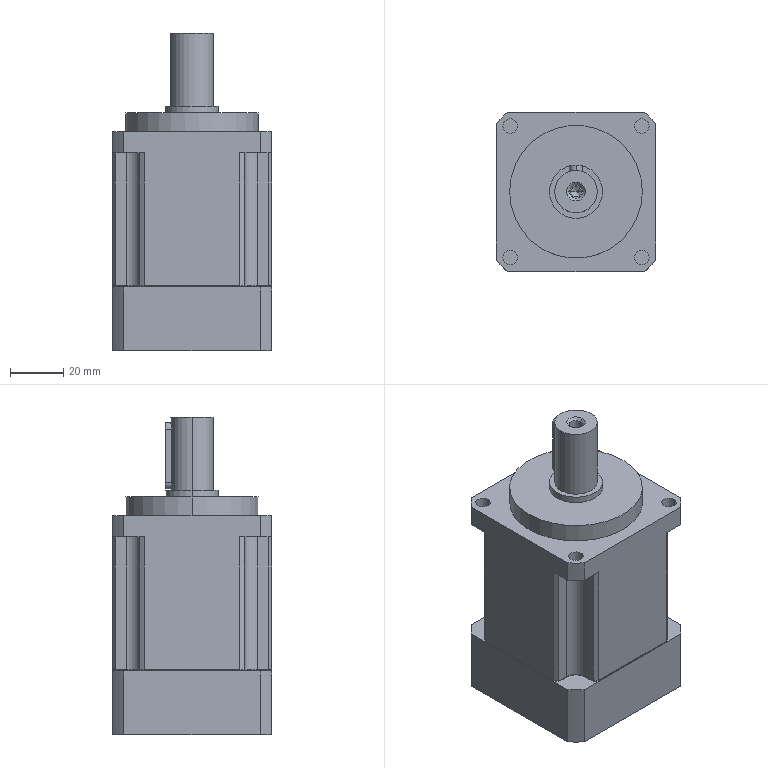Part | SolidWorks | features ICE 11, CirPattern 3, HoleWzd 2, Extrusion 1, Fillet 1 | 1 solid | 133 faces | box 60 x 60 x 119.5 mm | volume 279742 mm3 | cylinder 73 | plane 36 | cone 12 | torus 12 | commonest cylinder face diameters 5 x13 1 x12 4 x10 5.5 x8 70 x8 79 x8